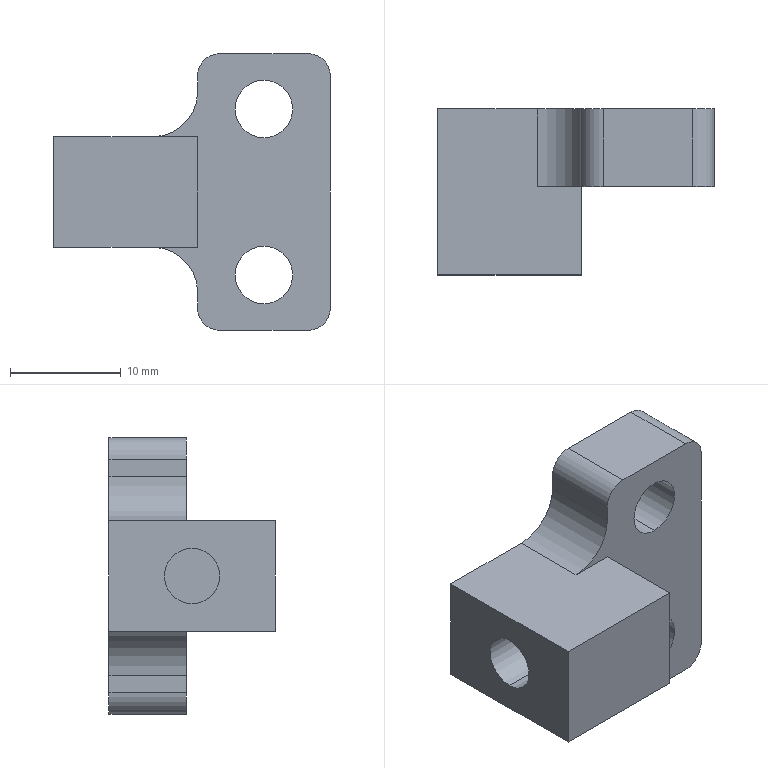NC program | Mastercam | posted with a generic post
Lines 1 to 20 of 16956:
%
O0000()
(MATERIAL - ALUMINUM MM - 2024)
( T24 | 63 FEM | H24 )
( T8 | 8 FEM | H8 )
( T6 | 6 FEM | H6 )
( T7 | 4 CHM | H7 )
N100 G21
N110 G0 G17 G40 G49 G80 G90
N120 T24 M6
N130 G0 G90 G54 X-86.8 Y0. A0. S4000 M3
N140 G43 H24 Z50. M8
N150 Z2.
N160 G1 Z0. F600.
N170 X86.8 F1000.
N180 G0 Z50.
N190 M5
N200 G91 G28 Z0. M9
N210 A0.
N220 M01